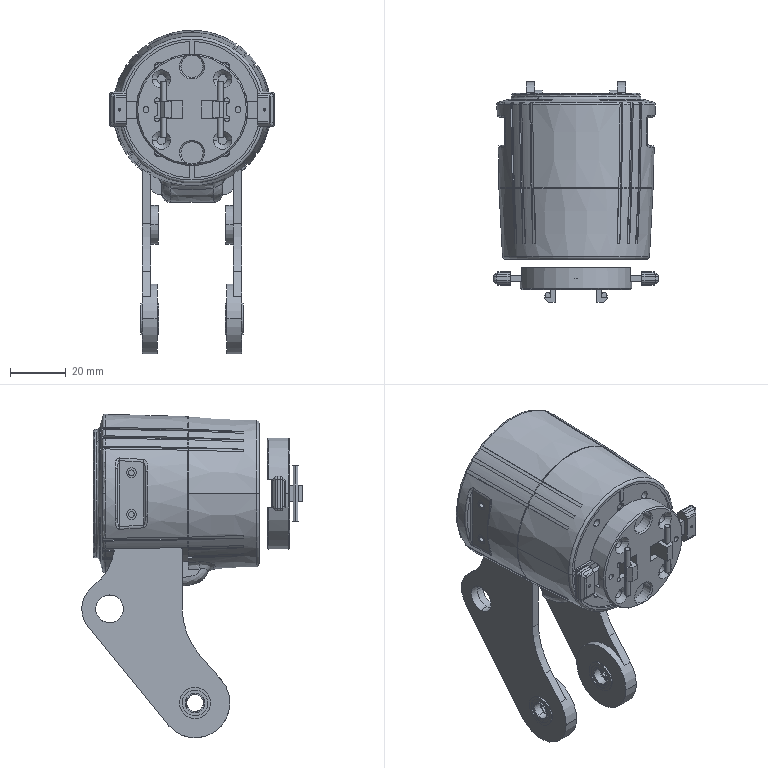Part | NX | features BREP 23, Delete Body 2, REPLACE_FACE 2, UNITE 1 | 26 solids | 1162 faces | box 59.043 x 79.079 x 115.958 mm | volume 60024 mm3 | plane 467 | cylinder 441 | cone 123 | torus 74 | spline 40 | sphere 17 | commonest cylinder face diameters 2 x84 3 x41 6 x21 0.8 x20 6.4 x20 10 x20